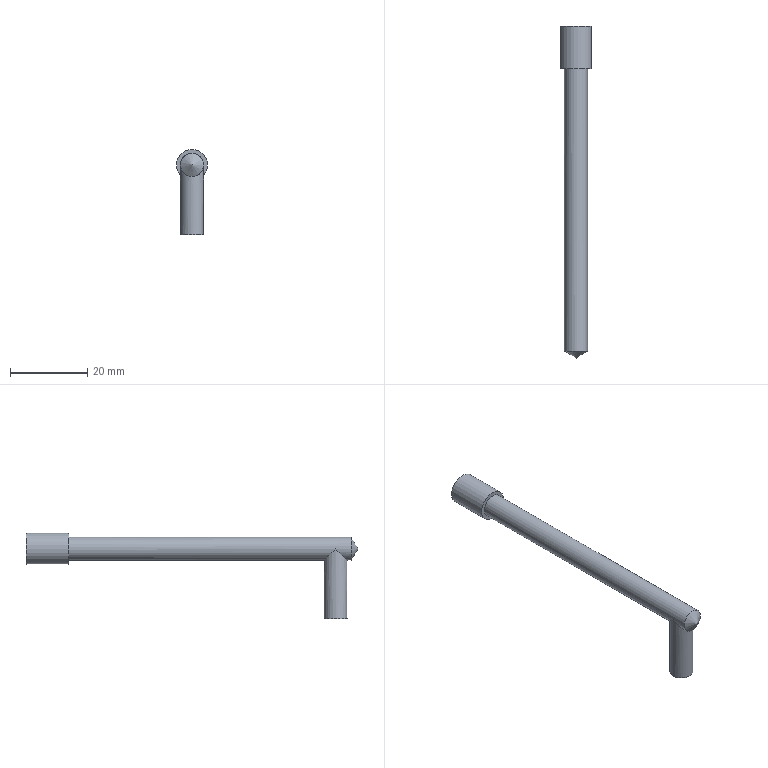Part | NX | features solid 2 | 1 solid | 7 faces | box 8 x 85.803 x 22 mm | volume 3071 mm3 | cylinder 3 | plane 3 | cone 1 | commonest cylinder face diameters 6 x2 8 x1
STEP:
#1=CARTESIAN_POINT('',(43.,30.,-52.));
#2=VERTEX_POINT('',#1);
#3=CARTESIAN_POINT('',(37.,30.,-52.));
#4=VERTEX_POINT('',#3);
#5=CARTESIAN_POINT('',(40.,30.,-52.));
#6=DIRECTION('',(0.,-0.7071,0.7071));
#7=DIRECTION('',(0.,-0.7071,-0.7071));
#8=AXIS2_PLACEMENT_3D('',#5,#6,#7);
#9=ELLIPSE('',#8,4.243,3.);
#10=EDGE_CURVE('',#2,#4,#9,.F.);
#11=ORIENTED_EDGE('',*,*,#10,.F.);
#12=CARTESIAN_POINT('',(40.,30.,-52.));
#13=DIRECTION('',(0.,-0.7071,-0.7071));
#14=DIRECTION('',(0.,-0.7071,0.7071));
#15=AXIS2_PLACEMENT_3D('',#12,#13,#14);
#16=ELLIPSE('',#15,4.243,3.);
#17=EDGE_CURVE('',#4,#2,#16,.T.);
#18=ORIENTED_EDGE('',*,*,#17,.F.);
#19=EDGE_LOOP('',(#11,#18));
#20=FACE_BOUND('',#19,.T.);
#21=CARTESIAN_POINT('',(40.,99.,-55.));
#22=VERTEX_POINT('',#21);
#23=CARTESIAN_POINT('',(40.,99.,-52.));
#24=DIRECTION('',(0.,-1.,0.));
#25=DIRECTION('',(0.,0.,-1.));
#26=AXIS2_PLACEMENT_3D('',#23,#24,#25);
#27=CIRCLE('',#26,3.);
#28=EDGE_CURVE('',#22,#22,#27,.F.);
#29=ORIENTED_EDGE('',*,*,#28,.F.);
#30=EDGE_LOOP('',(#29));
#31=FACE_BOUND('',#30,.T.);
#32=CARTESIAN_POINT('',(43.,26.,-52.));
#33=VERTEX_POINT('',#32);
#34=CARTESIAN_POINT('',(40.,26.,-52.));
#35=DIRECTION('',(0.,1.,0.));
#36=DIRECTION('',(1.,0.,0.));
#37=AXIS2_PLACEMENT_3D('',#34,#35,#36);
#38=CIRCLE('',#37,3.);
#39=EDGE_CURVE('',#33,#33,#38,.T.);
#40=ORIENTED_EDGE('',*,*,#39,.T.);
#41=EDGE_LOOP('',(#40));
#42=FACE_BOUND('',#41,.T.);
#43=CARTESIAN_POINT('',(40.,110.,-52.));
#44=DIRECTION('',(0.,-1.,0.));
#45=DIRECTION('',(1.,0.,0.));
#46=AXIS2_PLACEMENT_3D('',#43,#44,#45);
#47=CYLINDRICAL_SURFACE('',#46,3.);
#48=ADVANCED_FACE('',(#20,#31,#42),#47,.T.);
#49=ORIENTED_EDGE('',*,*,#39,.F.);
#50=EDGE_LOOP('',(#49));
#51=FACE_BOUND('',#50,.T.);
#52=CARTESIAN_POINT('',(40.,24.197,-52.));
#53=VERTEX_POINT('',#52);
#54=VERTEX_LOOP('',#53);
#55=FACE_BOUND('',#54,.T.);
#56=CARTESIAN_POINT('',(40.,24.197,-52.));
#57=DIRECTION('',(0.,1.,0.));
#58=DIRECTION('',(1.,0.,0.));
#59=AXIS2_PLACEMENT_3D('',#56,#57,#58);
#60=CONICAL_SURFACE('',#59,0.,1.03);
#61=ADVANCED_FACE('',(#51,#55),#60,.T.);
#62=ORIENTED_EDGE('',*,*,#28,.T.);
#63=EDGE_LOOP('',(#62));
#64=FACE_BOUND('',#63,.T.);
#65=CARTESIAN_POINT('',(44.,99.,-52.));
#66=VERTEX_POINT('',#65);
#67=CARTESIAN_POINT('',(40.,99.,-52.));
#68=DIRECTION('',(0.,1.,0.));
#69=DIRECTION('',(1.,0.,0.));
#70=AXIS2_PLACEMENT_3D('',#67,#68,#69);
#71=CIRCLE('',#70,4.);
#72=EDGE_CURVE('',#66,#66,#71,.T.);
#73=ORIENTED_EDGE('',*,*,#72,.F.);
#74=EDGE_LOOP('',(#73));
#75=FACE_BOUND('',#74,.T.);
#76=CARTESIAN_POINT('',(40.,99.,-52.));
#77=DIRECTION('',(0.,-1.,0.));
#78=DIRECTION('',(0.,0.,-1.));
#79=AXIS2_PLACEMENT_3D('',#76,#77,#78);
#80=PLANE('',#79);
#81=ADVANCED_FACE('',(#64,#75),#80,.T.);
#82=ORIENTED_EDGE('',*,*,#72,.T.);
#83=EDGE_LOOP('',(#82));
#84=FACE_BOUND('',#83,.T.);
#85=CARTESIAN_POINT('',(44.,110.,-52.));
#86=VERTEX_POINT('',#85);
#87=CARTESIAN_POINT('',(40.,110.,-52.));
#88=DIRECTION('',(0.,-1.,0.));
#89=DIRECTION('',(1.,0.,0.));
#90=AXIS2_PLACEMENT_3D('',#87,#88,#89);
#91=CIRCLE('',#90,4.);
#92=EDGE_CURVE('',#86,#86,#91,.T.);
#93=ORIENTED_EDGE('',*,*,#92,.T.);
#94=EDGE_LOOP('',(#93));
#95=FACE_BOUND('',#94,.T.);
#96=CARTESIAN_POINT('',(40.,110.,-52.));
#97=DIRECTION('',(0.,-1.,0.));
#98=DIRECTION('',(1.,0.,0.));
#99=AXIS2_PLACEMENT_3D('',#96,#97,#98);
#100=CYLINDRICAL_SURFACE('',#99,4.);
#101=ADVANCED_FACE('',(#84,#95),#100,.T.);
#102=ORIENTED_EDGE('',*,*,#92,.F.);
#103=EDGE_LOOP('',(#102));
#104=FACE_BOUND('',#103,.T.);
#105=CARTESIAN_POINT('',(40.,110.,-52.));
#106=DIRECTION('',(0.,1.,0.));
#107=DIRECTION('',(0.,0.,1.));
#108=AXIS2_PLACEMENT_3D('',#105,#106,#107);
#109=PLANE('',#108);
#110=ADVANCED_FACE('',(#104),#109,.T.);
#111=CARTESIAN_POINT('',(43.,30.,-70.));
#112=VERTEX_POINT('',#111);
#113=CARTESIAN_POINT('',(40.,30.,-70.));
#114=DIRECTION('',(0.,0.,1.));
#115=DIRECTION('',(1.,0.,0.));
#116=AXIS2_PLACEMENT_3D('',#113,#114,#115);
#117=CIRCLE('',#116,3.);
#118=EDGE_CURVE('',#112,#112,#117,.T.);
#119=ORIENTED_EDGE('',*,*,#118,.F.);
#120=EDGE_LOOP('',(#119));
#121=FACE_BOUND('',#120,.T.);
#122=CARTESIAN_POINT('',(40.,30.,-70.));
#123=DIRECTION('',(0.,0.,-1.));
#124=DIRECTION('',(-1.,0.,0.));
#125=AXIS2_PLACEMENT_3D('',#122,#123,#124);
#126=PLANE('',#125);
#127=ADVANCED_FACE('',(#121),#126,.T.);
#128=ORIENTED_EDGE('',*,*,#17,.T.);
#129=ORIENTED_EDGE('',*,*,#10,.T.);
#130=EDGE_LOOP('',(#128,#129));
#131=FACE_BOUND('',#130,.T.);
#132=ORIENTED_EDGE('',*,*,#118,.T.);
#133=EDGE_LOOP('',(#132));
#134=FACE_BOUND('',#133,.T.);
#135=CARTESIAN_POINT('',(40.,30.,-70.));
#136=DIRECTION('',(0.,0.,1.));
#137=DIRECTION('',(1.,0.,0.));
#138=AXIS2_PLACEMENT_3D('',#135,#136,#137);
#139=CYLINDRICAL_SURFACE('',#138,3.);
#140=ADVANCED_FACE('',(#131,#134),#139,.T.);
#141=CLOSED_SHELL('',(#48,#61,#81,#101,#110,#127,#140));
#142=MANIFOLD_SOLID_BREP('',#141);
#143=(LENGTH_UNIT()NAMED_UNIT(*)SI_UNIT(.MILLI.,.METRE.));
#144=UNCERTAINTY_MEASURE_WITH_UNIT(LENGTH_MEASURE(0.00001),#143,'','');
#145=(NAMED_UNIT(*)PLANE_ANGLE_UNIT()SI_UNIT($,.RADIAN.));
#146=(NAMED_UNIT(*)SI_UNIT($,.STERADIAN.)SOLID_ANGLE_UNIT());
#147=(GEOMETRIC_REPRESENTATION_CONTEXT(3)GLOBAL_UNCERTAINTY_ASSIGNED_CONTEXT((#144))GLOBAL_UNIT_ASSIGNED_CONTEXT((#143,#145,#146))REPRESENTATION_CONTEXT('',''));
#148=ADVANCED_BREP_SHAPE_REPRESENTATION('',(#142),#147);